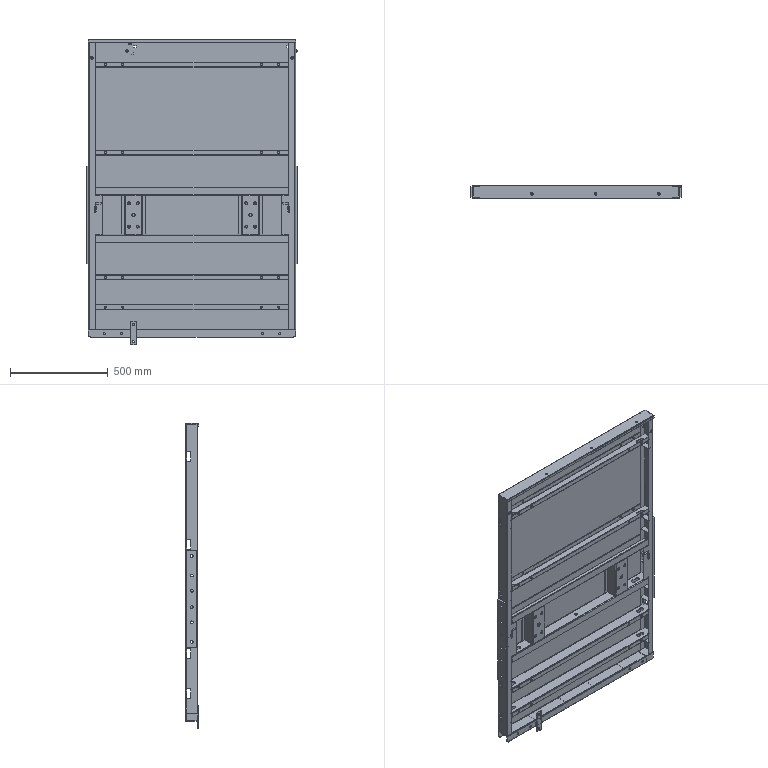Part | SolidWorks | features ReferencePattern 25, MirrorCompFeat 7, LocalLPattern 2 | 56 solids | 1606 faces | box 1080 x 70 x 1565 mm | volume 10438917 mm3 | plane 982 | cylinder 522 | cone 102 | commonest cylinder face diameters 10 x90 14.5 x88 11 x84 0.4 x36 8.4 x24 20 x24